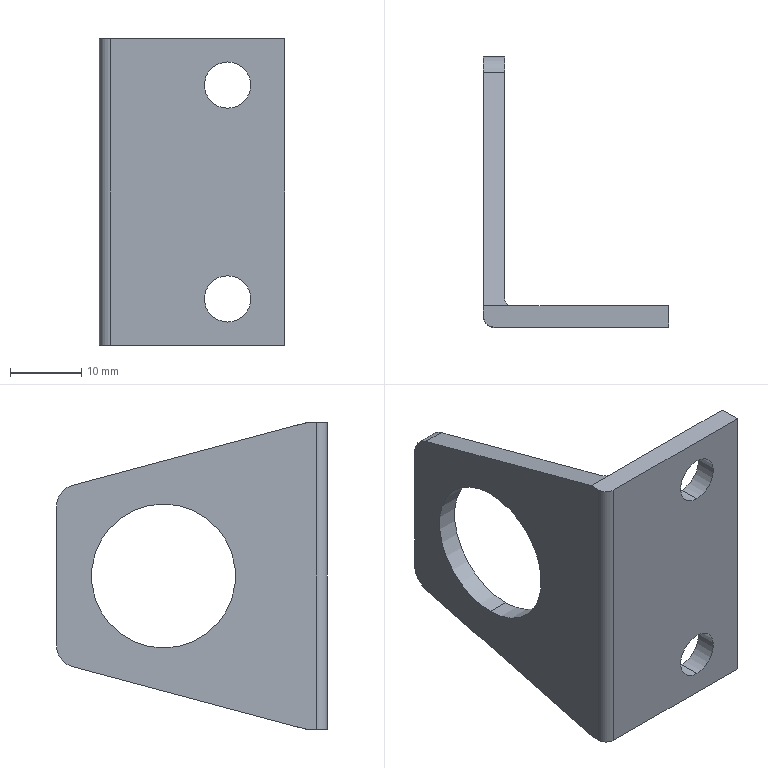Part | SolidWorks | features BaseBody 1 | 1 solid | 20 faces | box 26 x 38 x 43 mm | volume 5706 mm3 | cylinder 10 | plane 10 | commonest cylinder face diameters 6.5 x4 6 x2 20.2 x2 2 x1 3 x1
STEP:
#1=CARTESIAN_POINT('',(18.,0.,-11.75));
#2=VERTEX_POINT('',#1);
#3=CARTESIAN_POINT('',(18.,0.,-18.25));
#4=VERTEX_POINT('',#3);
#5=CARTESIAN_POINT('',(18.,0.,-15.));
#6=DIRECTION('',(0.,-1.,0.));
#7=DIRECTION('',(0.,0.,1.));
#8=AXIS2_PLACEMENT_3D('',#5,#6,#7);
#9=CIRCLE('',#8,3.25);
#10=EDGE_CURVE('',#2,#4,#9,.T.);
#11=ORIENTED_EDGE('',*,*,#10,.T.);
#12=CARTESIAN_POINT('',(18.,3.,-18.25));
#13=VERTEX_POINT('',#12);
#14=CARTESIAN_POINT('',(18.,3.,-18.25));
#15=DIRECTION('',(0.,1.,0.));
#16=VECTOR('',#15,1000.);
#17=LINE('',#14,#16);
#18=EDGE_CURVE('',#4,#13,#17,.T.);
#19=ORIENTED_EDGE('',*,*,#18,.T.);
#20=CARTESIAN_POINT('',(18.,3.,-11.75));
#21=VERTEX_POINT('',#20);
#22=CARTESIAN_POINT('',(18.,3.,-15.));
#23=DIRECTION('',(0.,-1.,0.));
#24=DIRECTION('',(0.,0.,1.));
#25=AXIS2_PLACEMENT_3D('',#22,#23,#24);
#26=CIRCLE('',#25,3.25);
#27=EDGE_CURVE('',#21,#13,#26,.T.);
#28=ORIENTED_EDGE('',*,*,#27,.F.);
#29=CARTESIAN_POINT('',(18.,3.,-11.75));
#30=DIRECTION('',(0.,1.,0.));
#31=VECTOR('',#30,1000.);
#32=LINE('',#29,#31);
#33=EDGE_CURVE('',#2,#21,#32,.T.);
#34=ORIENTED_EDGE('',*,*,#33,.F.);
#35=EDGE_LOOP('',(#11,#19,#28,#34));
#36=FACE_OUTER_BOUND('',#35,.T.);
#37=CARTESIAN_POINT('',(18.,3.,-15.));
#38=DIRECTION('',(0.,1.,0.));
#39=DIRECTION('',(0.,0.,1.));
#40=AXIS2_PLACEMENT_3D('',#37,#38,#39);
#41=CYLINDRICAL_SURFACE('',#40,3.25);
#42=ADVANCED_FACE('',(#36),#41,.F.);
#43=CARTESIAN_POINT('',(18.,0.,18.25));
#44=VERTEX_POINT('',#43);
#45=CARTESIAN_POINT('',(18.,0.,11.75));
#46=VERTEX_POINT('',#45);
#47=CARTESIAN_POINT('',(18.,0.,15.));
#48=DIRECTION('',(0.,-1.,0.));
#49=DIRECTION('',(0.,0.,1.));
#50=AXIS2_PLACEMENT_3D('',#47,#48,#49);
#51=CIRCLE('',#50,3.25);
#52=EDGE_CURVE('',#44,#46,#51,.T.);
#53=ORIENTED_EDGE('',*,*,#52,.T.);
#54=CARTESIAN_POINT('',(18.,3.,11.75));
#55=VERTEX_POINT('',#54);
#56=CARTESIAN_POINT('',(18.,3.,11.75));
#57=DIRECTION('',(0.,1.,0.));
#58=VECTOR('',#57,1000.);
#59=LINE('',#56,#58);
#60=EDGE_CURVE('',#46,#55,#59,.T.);
#61=ORIENTED_EDGE('',*,*,#60,.T.);
#62=CARTESIAN_POINT('',(18.,3.,18.25));
#63=VERTEX_POINT('',#62);
#64=CARTESIAN_POINT('',(18.,3.,15.));
#65=DIRECTION('',(0.,-1.,0.));
#66=DIRECTION('',(0.,0.,1.));
#67=AXIS2_PLACEMENT_3D('',#64,#65,#66);
#68=CIRCLE('',#67,3.25);
#69=EDGE_CURVE('',#63,#55,#68,.T.);
#70=ORIENTED_EDGE('',*,*,#69,.F.);
#71=CARTESIAN_POINT('',(18.,3.,18.25));
#72=DIRECTION('',(0.,1.,0.));
#73=VECTOR('',#72,1000.);
#74=LINE('',#71,#73);
#75=EDGE_CURVE('',#44,#63,#74,.T.);
#76=ORIENTED_EDGE('',*,*,#75,.F.);
#77=EDGE_LOOP('',(#53,#61,#70,#76));
#78=FACE_OUTER_BOUND('',#77,.T.);
#79=CARTESIAN_POINT('',(18.,3.,15.));
#80=DIRECTION('',(0.,1.,0.));
#81=DIRECTION('',(0.,0.,1.));
#82=AXIS2_PLACEMENT_3D('',#79,#80,#81);
#83=CYLINDRICAL_SURFACE('',#82,3.25);
#84=ADVANCED_FACE('',(#78),#83,.F.);
#85=CARTESIAN_POINT('',(0.,23.,-10.1));
#86=VERTEX_POINT('',#85);
#87=CARTESIAN_POINT('',(0.,23.,10.1));
#88=VERTEX_POINT('',#87);
#89=CARTESIAN_POINT('',(0.,23.,0.));
#90=DIRECTION('',(-1.,0.,0.));
#91=DIRECTION('',(0.,0.,-1.));
#92=AXIS2_PLACEMENT_3D('',#89,#90,#91);
#93=CIRCLE('',#92,10.1);
#94=EDGE_CURVE('',#86,#88,#93,.T.);
#95=ORIENTED_EDGE('',*,*,#94,.T.);
#96=CARTESIAN_POINT('',(3.,23.,10.1));
#97=VERTEX_POINT('',#96);
#98=CARTESIAN_POINT('',(26.,23.,10.1));
#99=DIRECTION('',(1.,0.,0.));
#100=VECTOR('',#99,1000.);
#101=LINE('',#98,#100);
#102=EDGE_CURVE('',#88,#97,#101,.T.);
#103=ORIENTED_EDGE('',*,*,#102,.T.);
#104=CARTESIAN_POINT('',(3.,23.,-10.1));
#105=VERTEX_POINT('',#104);
#106=CARTESIAN_POINT('',(3.,23.,0.));
#107=DIRECTION('',(-1.,0.,0.));
#108=DIRECTION('',(0.,0.,-1.));
#109=AXIS2_PLACEMENT_3D('',#106,#107,#108);
#110=CIRCLE('',#109,10.1);
#111=EDGE_CURVE('',#105,#97,#110,.T.);
#112=ORIENTED_EDGE('',*,*,#111,.F.);
#113=CARTESIAN_POINT('',(26.,23.,-10.1));
#114=DIRECTION('',(1.,0.,0.));
#115=VECTOR('',#114,1000.);
#116=LINE('',#113,#115);
#117=EDGE_CURVE('',#86,#105,#116,.T.);
#118=ORIENTED_EDGE('',*,*,#117,.F.);
#119=EDGE_LOOP('',(#95,#103,#112,#118));
#120=FACE_OUTER_BOUND('',#119,.T.);
#121=CARTESIAN_POINT('',(26.,23.,0.));
#122=DIRECTION('',(1.,0.,0.));
#123=DIRECTION('',(0.,0.,-1.));
#124=AXIS2_PLACEMENT_3D('',#121,#122,#123);
#125=CYLINDRICAL_SURFACE('',#124,10.1);
#126=ADVANCED_FACE('',(#120),#125,.F.);
#127=CARTESIAN_POINT('',(26.,0.,-21.5));
#128=VERTEX_POINT('',#127);
#129=CARTESIAN_POINT('',(1.5,0.,-21.5));
#130=VERTEX_POINT('',#129);
#131=CARTESIAN_POINT('',(26.,0.,-21.5));
#132=DIRECTION('',(-1.,0.,0.));
#133=VECTOR('',#132,1000.);
#134=LINE('',#131,#133);
#135=EDGE_CURVE('',#128,#130,#134,.T.);
#136=ORIENTED_EDGE('',*,*,#135,.F.);
#137=CARTESIAN_POINT('',(26.,0.,21.5));
#138=VERTEX_POINT('',#137);
#139=CARTESIAN_POINT('',(26.,0.,21.5));
#140=DIRECTION('',(0.,0.,-1.));
#141=VECTOR('',#140,1000.);
#142=LINE('',#139,#141);
#143=EDGE_CURVE('',#138,#128,#142,.T.);
#144=ORIENTED_EDGE('',*,*,#143,.F.);
#145=CARTESIAN_POINT('',(1.5,0.,21.5));
#146=VERTEX_POINT('',#145);
#147=CARTESIAN_POINT('',(26.,0.,21.5));
#148=DIRECTION('',(1.,0.,0.));
#149=VECTOR('',#148,1000.);
#150=LINE('',#147,#149);
#151=EDGE_CURVE('',#146,#138,#150,.T.);
#152=ORIENTED_EDGE('',*,*,#151,.F.);
#153=CARTESIAN_POINT('',(1.5,0.,21.5));
#154=DIRECTION('',(0.,0.,1.));
#155=VECTOR('',#154,1000.);
#156=LINE('',#153,#155);
#157=EDGE_CURVE('',#130,#146,#156,.T.);
#158=ORIENTED_EDGE('',*,*,#157,.F.);
#159=EDGE_LOOP('',(#136,#144,#152,#158));
#160=FACE_OUTER_BOUND('',#159,.T.);
#161=ORIENTED_EDGE('',*,*,#10,.F.);
#162=CARTESIAN_POINT('',(18.,0.,-15.));
#163=DIRECTION('',(0.,-1.,0.));
#164=DIRECTION('',(0.,0.,1.));
#165=AXIS2_PLACEMENT_3D('',#162,#163,#164);
#166=CIRCLE('',#165,3.25);
#167=EDGE_CURVE('',#4,#2,#166,.T.);
#168=ORIENTED_EDGE('',*,*,#167,.F.);
#169=EDGE_LOOP('',(#161,#168));
#170=FACE_BOUND('',#169,.T.);
#171=ORIENTED_EDGE('',*,*,#52,.F.);
#172=CARTESIAN_POINT('',(18.,0.,15.));
#173=DIRECTION('',(0.,-1.,0.));
#174=DIRECTION('',(0.,0.,1.));
#175=AXIS2_PLACEMENT_3D('',#172,#173,#174);
#176=CIRCLE('',#175,3.25);
#177=EDGE_CURVE('',#46,#44,#176,.T.);
#178=ORIENTED_EDGE('',*,*,#177,.F.);
#179=EDGE_LOOP('',(#171,#178));
#180=FACE_BOUND('',#179,.T.);
#181=CARTESIAN_POINT('',(26.,0.,21.5));
#182=DIRECTION('',(0.,1.,0.));
#183=DIRECTION('',(0.,0.,1.));
#184=AXIS2_PLACEMENT_3D('',#181,#182,#183);
#185=PLANE('',#184);
#186=ADVANCED_FACE('',(#160,#170,#180),#185,.F.);
#187=CARTESIAN_POINT('',(0.,1.5,21.5));
#188=VERTEX_POINT('',#187);
#189=CARTESIAN_POINT('',(1.5,1.5,21.5));
#190=DIRECTION('',(0.,0.,-1.));
#191=DIRECTION('',(1.,0.,0.));
#192=AXIS2_PLACEMENT_3D('',#189,#190,#191);
#193=CIRCLE('',#192,1.5);
#194=EDGE_CURVE('',#146,#188,#193,.T.);
#195=ORIENTED_EDGE('',*,*,#194,.T.);
#196=CARTESIAN_POINT('',(0.,1.5,-21.5));
#197=VERTEX_POINT('',#196);
#198=CARTESIAN_POINT('',(0.,1.5,21.5));
#199=DIRECTION('',(0.,0.,-1.));
#200=VECTOR('',#199,1000.);
#201=LINE('',#198,#200);
#202=EDGE_CURVE('',#188,#197,#201,.T.);
#203=ORIENTED_EDGE('',*,*,#202,.T.);
#204=CARTESIAN_POINT('',(1.5,1.5,-21.5));
#205=DIRECTION('',(0.,0.,1.));
#206=DIRECTION('',(1.,0.,0.));
#207=AXIS2_PLACEMENT_3D('',#204,#205,#206);
#208=CIRCLE('',#207,1.5);
#209=EDGE_CURVE('',#197,#130,#208,.T.);
#210=ORIENTED_EDGE('',*,*,#209,.T.);
#211=ORIENTED_EDGE('',*,*,#157,.T.);
#212=EDGE_LOOP('',(#195,#203,#210,#211));
#213=FACE_OUTER_BOUND('',#212,.T.);
#214=CARTESIAN_POINT('',(1.5,1.5,21.5));
#215=DIRECTION('',(0.,0.,1.));
#216=DIRECTION('',(1.,0.,0.));
#217=AXIS2_PLACEMENT_3D('',#214,#215,#216);
#218=CYLINDRICAL_SURFACE('',#217,1.5);
#219=ADVANCED_FACE('',(#213),#218,.T.);
#220=ORIENTED_EDGE('',*,*,#209,.F.);
#221=CARTESIAN_POINT('',(0.,3.,-21.5));
#222=VERTEX_POINT('',#221);
#223=CARTESIAN_POINT('',(0.,0.,-21.5));
#224=DIRECTION('',(0.,-1.,0.));
#225=VECTOR('',#224,1000.);
#226=LINE('',#223,#225);
#227=EDGE_CURVE('',#222,#197,#226,.T.);
#228=ORIENTED_EDGE('',*,*,#227,.F.);
#229=CARTESIAN_POINT('',(4.,3.,-21.5));
#230=VERTEX_POINT('',#229);
#231=CARTESIAN_POINT('',(26.,3.,-21.5));
#232=DIRECTION('',(-1.,0.,0.));
#233=VECTOR('',#232,1000.);
#234=LINE('',#231,#233);
#235=EDGE_CURVE('',#230,#222,#234,.T.);
#236=ORIENTED_EDGE('',*,*,#235,.F.);
#237=CARTESIAN_POINT('',(26.,3.,-21.5));
#238=VERTEX_POINT('',#237);
#239=CARTESIAN_POINT('',(26.,3.,-21.5));
#240=DIRECTION('',(-1.,0.,0.));
#241=VECTOR('',#240,1000.);
#242=LINE('',#239,#241);
#243=EDGE_CURVE('',#238,#230,#242,.T.);
#244=ORIENTED_EDGE('',*,*,#243,.F.);
#245=CARTESIAN_POINT('',(26.,0.,-21.5));
#246=DIRECTION('',(0.,1.,0.));
#247=VECTOR('',#246,1000.);
#248=LINE('',#245,#247);
#249=EDGE_CURVE('',#128,#238,#248,.T.);
#250=ORIENTED_EDGE('',*,*,#249,.F.);
#251=ORIENTED_EDGE('',*,*,#135,.T.);
#252=EDGE_LOOP('',(#220,#228,#236,#244,#250,#251));
#253=FACE_OUTER_BOUND('',#252,.T.);
#254=CARTESIAN_POINT('',(26.,0.,-21.5));
#255=DIRECTION('',(0.,0.,1.));
#256=DIRECTION('',(0.,-1.,0.));
#257=AXIS2_PLACEMENT_3D('',#254,#255,#256);
#258=PLANE('',#257);
#259=ADVANCED_FACE('',(#253),#258,.F.);
#260=CARTESIAN_POINT('',(26.,3.,21.5));
#261=VERTEX_POINT('',#260);
#262=CARTESIAN_POINT('',(26.,35.,21.5));
#263=DIRECTION('',(0.,-1.,0.));
#264=VECTOR('',#263,1000.);
#265=LINE('',#262,#264);
#266=EDGE_CURVE('',#261,#138,#265,.T.);
#267=ORIENTED_EDGE('',*,*,#266,.T.);
#268=ORIENTED_EDGE('',*,*,#143,.T.);
#269=ORIENTED_EDGE('',*,*,#249,.T.);
#270=CARTESIAN_POINT('',(26.,3.,-9.82));
#271=DIRECTION('',(0.,0.,1.));
#272=VECTOR('',#271,1000.);
#273=LINE('',#270,#272);
#274=EDGE_CURVE('',#238,#261,#273,.T.);
#275=ORIENTED_EDGE('',*,*,#274,.T.);
#276=EDGE_LOOP('',(#267,#268,#269,#275));
#277=FACE_OUTER_BOUND('',#276,.T.);
#278=CARTESIAN_POINT('',(26.,35.,-9.82));
#279=DIRECTION('',(1.,0.,0.));
#280=DIRECTION('',(0.,0.,-1.));
#281=AXIS2_PLACEMENT_3D('',#278,#279,#280);
#282=PLANE('',#281);
#283=ADVANCED_FACE('',(#277),#282,.T.);
#284=ORIENTED_EDGE('',*,*,#194,.F.);
#285=ORIENTED_EDGE('',*,*,#151,.T.);
#286=ORIENTED_EDGE('',*,*,#266,.F.);
#287=CARTESIAN_POINT('',(4.,3.,21.5));
#288=VERTEX_POINT('',#287);
#289=CARTESIAN_POINT('',(26.,3.,21.5));
#290=DIRECTION('',(1.,0.,0.));
#291=VECTOR('',#290,1000.);
#292=LINE('',#289,#291);
#293=EDGE_CURVE('',#288,#261,#292,.T.);
#294=ORIENTED_EDGE('',*,*,#293,.F.);
#295=CARTESIAN_POINT('',(0.,3.,21.5));
#296=VERTEX_POINT('',#295);
#297=CARTESIAN_POINT('',(26.,3.,21.5));
#298=DIRECTION('',(1.,0.,0.));
#299=VECTOR('',#298,1000.);
#300=LINE('',#297,#299);
#301=EDGE_CURVE('',#296,#288,#300,.T.);
#302=ORIENTED_EDGE('',*,*,#301,.F.);
#303=CARTESIAN_POINT('',(0.,3.,21.5));
#304=DIRECTION('',(0.,1.,0.));
#305=VECTOR('',#304,1000.);
#306=LINE('',#303,#305);
#307=EDGE_CURVE('',#188,#296,#306,.T.);
#308=ORIENTED_EDGE('',*,*,#307,.F.);
#309=EDGE_LOOP('',(#284,#285,#286,#294,#302,#308));
#310=FACE_OUTER_BOUND('',#309,.T.);
#311=CARTESIAN_POINT('',(26.,3.,21.5));
#312=DIRECTION('',(0.,0.,-1.));
#313=DIRECTION('',(-1.,0.,0.));
#314=AXIS2_PLACEMENT_3D('',#311,#312,#313);
#315=PLANE('',#314);
#316=ADVANCED_FACE('',(#310),#315,.F.);
#317=ORIENTED_EDGE('',*,*,#18,.F.);
#318=ORIENTED_EDGE('',*,*,#167,.T.);
#319=ORIENTED_EDGE('',*,*,#33,.T.);
#320=CARTESIAN_POINT('',(18.,3.,-15.));
#321=DIRECTION('',(0.,-1.,0.));
#322=DIRECTION('',(0.,0.,1.));
#323=AXIS2_PLACEMENT_3D('',#320,#321,#322);
#324=CIRCLE('',#323,3.25);
#325=EDGE_CURVE('',#13,#21,#324,.T.);
#326=ORIENTED_EDGE('',*,*,#325,.F.);
#327=EDGE_LOOP('',(#317,#318,#319,#326));
#328=FACE_OUTER_BOUND('',#327,.T.);
#329=CARTESIAN_POINT('',(18.,3.,-15.));
#330=DIRECTION('',(0.,1.,0.));
#331=DIRECTION('',(0.,0.,1.));
#332=AXIS2_PLACEMENT_3D('',#329,#330,#331);
#333=CYLINDRICAL_SURFACE('',#332,3.25);
#334=ADVANCED_FACE('',(#328),#333,.F.);
#335=ORIENTED_EDGE('',*,*,#60,.F.);
#336=ORIENTED_EDGE('',*,*,#177,.T.);
#337=ORIENTED_EDGE('',*,*,#75,.T.);
#338=CARTESIAN_POINT('',(18.,3.,15.));
#339=DIRECTION('',(0.,-1.,0.));
#340=DIRECTION('',(0.,0.,1.));
#341=AXIS2_PLACEMENT_3D('',#338,#339,#340);
#342=CIRCLE('',#341,3.25);
#343=EDGE_CURVE('',#55,#63,#342,.T.);
#344=ORIENTED_EDGE('',*,*,#343,.F.);
#345=EDGE_LOOP('',(#335,#336,#337,#344));
#346=FACE_OUTER_BOUND('',#345,.T.);
#347=CARTESIAN_POINT('',(18.,3.,15.));
#348=DIRECTION('',(0.,1.,0.));
#349=DIRECTION('',(0.,0.,1.));
#350=AXIS2_PLACEMENT_3D('',#347,#348,#349);
#351=CYLINDRICAL_SURFACE('',#350,3.25);
#352=ADVANCED_FACE('',(#346),#351,.F.);
#353=ORIENTED_EDGE('',*,*,#202,.F.);
#354=ORIENTED_EDGE('',*,*,#307,.T.);
#355=CARTESIAN_POINT('',(0.,35.776,12.718));
#356=VERTEX_POINT('',#355);
#357=CARTESIAN_POINT('',(0.,35.776,12.718));
#358=DIRECTION('',(0.,-0.9659,0.2588));
#359=VECTOR('',#358,1000.);
#360=LINE('',#357,#359);
#361=EDGE_CURVE('',#356,#296,#360,.T.);
#362=ORIENTED_EDGE('',*,*,#361,.F.);
#363=CARTESIAN_POINT('',(0.,38.,9.82));
#364=VERTEX_POINT('',#363);
#365=CARTESIAN_POINT('',(0.,35.,9.82));
#366=DIRECTION('',(1.,0.,0.));
#367=DIRECTION('',(0.,0.,-1.));
#368=AXIS2_PLACEMENT_3D('',#365,#366,#367);
#369=CIRCLE('',#368,3.);
#370=EDGE_CURVE('',#364,#356,#369,.T.);
#371=ORIENTED_EDGE('',*,*,#370,.F.);
#372=CARTESIAN_POINT('',(0.,38.,-9.82));
#373=VERTEX_POINT('',#372);
#374=CARTESIAN_POINT('',(0.,38.,-9.82));
#375=DIRECTION('',(0.,0.,1.));
#376=VECTOR('',#375,1000.);
#377=LINE('',#374,#376);
#378=EDGE_CURVE('',#373,#364,#377,.T.);
#379=ORIENTED_EDGE('',*,*,#378,.F.);
#380=CARTESIAN_POINT('',(0.,35.776,-12.718));
#381=VERTEX_POINT('',#380);
#382=CARTESIAN_POINT('',(0.,35.,-9.82));
#383=DIRECTION('',(1.,0.,0.));
#384=DIRECTION('',(0.,0.,-1.));
#385=AXIS2_PLACEMENT_3D('',#382,#383,#384);
#386=CIRCLE('',#385,3.);
#387=EDGE_CURVE('',#381,#373,#386,.T.);
#388=ORIENTED_EDGE('',*,*,#387,.F.);
#389=CARTESIAN_POINT('',(0.,3.,-21.5));
#390=DIRECTION('',(0.,0.9659,0.2588));
#391=VECTOR('',#390,1000.);
#392=LINE('',#389,#391);
#393=EDGE_CURVE('',#222,#381,#392,.T.);
#394=ORIENTED_EDGE('',*,*,#393,.F.);
#395=ORIENTED_EDGE('',*,*,#227,.T.);
#396=EDGE_LOOP('',(#353,#354,#362,#371,#379,#388,#394,#395));
#397=FACE_OUTER_BOUND('',#396,.T.);
#398=ORIENTED_EDGE('',*,*,#94,.F.);
#399=CARTESIAN_POINT('',(0.,23.,0.));
#400=DIRECTION('',(-1.,0.,0.));
#401=DIRECTION('',(0.,0.,-1.));
#402=AXIS2_PLACEMENT_3D('',#399,#400,#401);
#403=CIRCLE('',#402,10.1);
#404=EDGE_CURVE('',#88,#86,#403,.T.);
#405=ORIENTED_EDGE('',*,*,#404,.F.);
#406=EDGE_LOOP('',(#398,#405));
#407=FACE_BOUND('',#406,.T.);
#408=CARTESIAN_POINT('',(0.,35.,-9.82));
#409=DIRECTION('',(1.,0.,0.));
#410=DIRECTION('',(0.,0.,-1.));
#411=AXIS2_PLACEMENT_3D('',#408,#409,#410);
#412=PLANE('',#411);
#413=ADVANCED_FACE('',(#397,#407),#412,.F.);
#414=CARTESIAN_POINT('',(3.,4.,-21.232));
#415=VERTEX_POINT('',#414);
#416=CARTESIAN_POINT('',(3.,4.,-21.232));
#417=CARTESIAN_POINT('',(3.,3.414,-21.389));
#418=CARTESIAN_POINT('',(3.414,3.,-21.5));
#419=CARTESIAN_POINT('',(4.,3.,-21.5));
#420=(BOUNDED_CURVE()B_SPLINE_CURVE(3,(#416,#417,#418,#419),.UNSPECIFIED.,.F.,.F.)B_SPLINE_CURVE_WITH_KNOTS((4,4),(1.571,3.142),.UNSPECIFIED.)CURVE()GEOMETRIC_REPRESENTATION_ITEM()RATIONAL_B_SPLINE_CURVE((1.,0.8047,0.8047,1.))REPRESENTATION_ITEM(''));
#421=EDGE_CURVE('',#415,#230,#420,.T.);
#422=ORIENTED_EDGE('',*,*,#421,.T.);
#423=ORIENTED_EDGE('',*,*,#235,.T.);
#424=ORIENTED_EDGE('',*,*,#393,.T.);
#425=CARTESIAN_POINT('',(3.,35.776,-12.718));
#426=VERTEX_POINT('',#425);
#427=CARTESIAN_POINT('',(26.,35.776,-12.718));
#428=DIRECTION('',(-1.,0.,0.));
#429=VECTOR('',#428,1000.);
#430=LINE('',#427,#429);
#431=EDGE_CURVE('',#426,#381,#430,.T.);
#432=ORIENTED_EDGE('',*,*,#431,.F.);
#433=CARTESIAN_POINT('',(3.,3.,-21.5));
#434=DIRECTION('',(0.,0.9659,0.2588));
#435=VECTOR('',#434,1000.);
#436=LINE('',#433,#435);
#437=EDGE_CURVE('',#415,#426,#436,.T.);
#438=ORIENTED_EDGE('',*,*,#437,.F.);
#439=EDGE_LOOP('',(#422,#423,#424,#432,#438));
#440=FACE_OUTER_BOUND('',#439,.T.);
#441=CARTESIAN_POINT('',(26.,3.,-21.5));
#442=DIRECTION('',(0.,-0.2588,0.9659));
#443=DIRECTION('',(0.,-0.9659,-0.2588));
#444=AXIS2_PLACEMENT_3D('',#441,#442,#443);
#445=PLANE('',#444);
#446=ADVANCED_FACE('',(#440),#445,.F.);
#447=ORIENTED_EDGE('',*,*,#293,.T.);
#448=ORIENTED_EDGE('',*,*,#274,.F.);
#449=ORIENTED_EDGE('',*,*,#243,.T.);
#450=CARTESIAN_POINT('',(4.,3.,21.5));
#451=DIRECTION('',(0.,0.,1.));
#452=VECTOR('',#451,1000.);
#453=LINE('',#450,#452);
#454=EDGE_CURVE('',#230,#288,#453,.T.);
#455=ORIENTED_EDGE('',*,*,#454,.T.);
#456=EDGE_LOOP('',(#447,#448,#449,#455));
#457=FACE_OUTER_BOUND('',#456,.T.);
#458=ORIENTED_EDGE('',*,*,#27,.T.);
#459=ORIENTED_EDGE('',*,*,#325,.T.);
#460=EDGE_LOOP('',(#458,#459));
#461=FACE_BOUND('',#460,.T.);
#462=ORIENTED_EDGE('',*,*,#69,.T.);
#463=ORIENTED_EDGE('',*,*,#343,.T.);
#464=EDGE_LOOP('',(#462,#463));
#465=FACE_BOUND('',#464,.T.);
#466=CARTESIAN_POINT('',(4.,3.,21.5));
#467=DIRECTION('',(0.,1.,0.));
#468=DIRECTION('',(0.,0.,1.));
#469=AXIS2_PLACEMENT_3D('',#466,#467,#468);
#470=PLANE('',#469);
#471=ADVANCED_FACE('',(#457,#461,#465),#470,.T.);
#472=CARTESIAN_POINT('',(3.,35.776,12.718));
#473=VERTEX_POINT('',#472);
#474=CARTESIAN_POINT('',(26.,35.776,12.718));
#475=DIRECTION('',(1.,0.,0.));
#476=VECTOR('',#475,1000.);
#477=LINE('',#474,#476);
#478=EDGE_CURVE('',#356,#473,#477,.T.);
#479=ORIENTED_EDGE('',*,*,#478,.F.);
#480=ORIENTED_EDGE('',*,*,#361,.T.);
#481=ORIENTED_EDGE('',*,*,#301,.T.);
#482=CARTESIAN_POINT('',(3.,4.,21.232));
#483=VERTEX_POINT('',#482);
#484=CARTESIAN_POINT('',(3.,4.,21.232));
#485=CARTESIAN_POINT('',(3.,3.414,21.389));
#486=CARTESIAN_POINT('',(3.414,3.,21.5));
#487=CARTESIAN_POINT('',(4.,3.,21.5));
#488=(BOUNDED_CURVE()B_SPLINE_CURVE(3,(#484,#485,#486,#487),.UNSPECIFIED.,.F.,.F.)B_SPLINE_CURVE_WITH_KNOTS((4,4),(4.712,6.283),.UNSPECIFIED.)CURVE()GEOMETRIC_REPRESENTATION_ITEM()RATIONAL_B_SPLINE_CURVE((1.,0.8047,0.8047,1.))REPRESENTATION_ITEM(''));
#489=EDGE_CURVE('',#483,#288,#488,.T.);
#490=ORIENTED_EDGE('',*,*,#489,.F.);
#491=CARTESIAN_POINT('',(3.,35.776,12.718));
#492=DIRECTION('',(0.,-0.9659,0.2588));
#493=VECTOR('',#492,1000.);
#494=LINE('',#491,#493);
#495=EDGE_CURVE('',#473,#483,#494,.T.);
#496=ORIENTED_EDGE('',*,*,#495,.F.);
#497=EDGE_LOOP('',(#479,#480,#481,#490,#496));
#498=FACE_OUTER_BOUND('',#497,.T.);
#499=CARTESIAN_POINT('',(26.,35.776,12.718));
#500=DIRECTION('',(0.,-0.2588,-0.9659));
#501=DIRECTION('',(0.,0.9659,-0.2588));
#502=AXIS2_PLACEMENT_3D('',#499,#500,#501);
#503=PLANE('',#502);
#504=ADVANCED_FACE('',(#498),#503,.F.);
#505=ORIENTED_EDGE('',*,*,#370,.T.);
#506=ORIENTED_EDGE('',*,*,#478,.T.);
#507=CARTESIAN_POINT('',(3.,38.,9.82));
#508=VERTEX_POINT('',#507);
#509=CARTESIAN_POINT('',(3.,35.,9.82));
#510=DIRECTION('',(-1.,0.,0.));
#511=DIRECTION('',(0.,0.,-1.));
#512=AXIS2_PLACEMENT_3D('',#509,#510,#511);
#513=CIRCLE('',#512,3.);
#514=EDGE_CURVE('',#473,#508,#513,.T.);
#515=ORIENTED_EDGE('',*,*,#514,.T.);
#516=CARTESIAN_POINT('',(26.,38.,9.82));
#517=DIRECTION('',(-1.,0.,0.));
#518=VECTOR('',#517,1000.);
#519=LINE('',#516,#518);
#520=EDGE_CURVE('',#508,#364,#519,.T.);
#521=ORIENTED_EDGE('',*,*,#520,.T.);
#522=EDGE_LOOP('',(#505,#506,#515,#521));
#523=FACE_OUTER_BOUND('',#522,.T.);
#524=CARTESIAN_POINT('',(26.,35.,9.82));
#525=DIRECTION('',(1.,0.,0.));
#526=DIRECTION('',(0.,0.,-1.));
#527=AXIS2_PLACEMENT_3D('',#524,#525,#526);
#528=CYLINDRICAL_SURFACE('',#527,3.);
#529=ADVANCED_FACE('',(#523),#528,.T.);
#530=CARTESIAN_POINT('',(3.,38.,-9.82));
#531=VERTEX_POINT('',#530);
#532=CARTESIAN_POINT('',(26.,38.,-9.82));
#533=DIRECTION('',(1.,0.,0.));
#534=VECTOR('',#533,1000.);
#535=LINE('',#532,#534);
#536=EDGE_CURVE('',#373,#531,#535,.T.);
#537=ORIENTED_EDGE('',*,*,#536,.F.);
#538=ORIENTED_EDGE('',*,*,#378,.T.);
#539=ORIENTED_EDGE('',*,*,#520,.F.);
#540=CARTESIAN_POINT('',(3.,38.,-9.82));
#541=DIRECTION('',(0.,0.,1.));
#542=VECTOR('',#541,1000.);
#543=LINE('',#540,#542);
#544=EDGE_CURVE('',#531,#508,#543,.T.);
#545=ORIENTED_EDGE('',*,*,#544,.F.);
#546=EDGE_LOOP('',(#537,#538,#539,#545));
#547=FACE_OUTER_BOUND('',#546,.T.);
#548=CARTESIAN_POINT('',(26.,38.,-9.82));
#549=DIRECTION('',(0.,-1.,0.));
#550=DIRECTION('',(0.,0.,-1.));
#551=AXIS2_PLACEMENT_3D('',#548,#549,#550);
#552=PLANE('',#551);
#553=ADVANCED_FACE('',(#547),#552,.F.);
#554=ORIENTED_EDGE('',*,*,#387,.T.);
#555=ORIENTED_EDGE('',*,*,#536,.T.);
#556=CARTESIAN_POINT('',(3.,35.,-9.82));
#557=DIRECTION('',(-1.,0.,0.));
#558=DIRECTION('',(0.,0.,-1.));
#559=AXIS2_PLACEMENT_3D('',#556,#557,#558);
#560=CIRCLE('',#559,3.);
#561=EDGE_CURVE('',#531,#426,#560,.T.);
#562=ORIENTED_EDGE('',*,*,#561,.T.);
#563=ORIENTED_EDGE('',*,*,#431,.T.);
#564=EDGE_LOOP('',(#554,#555,#562,#563));
#565=FACE_OUTER_BOUND('',#564,.T.);
#566=CARTESIAN_POINT('',(26.,35.,-9.82));
#567=DIRECTION('',(1.,0.,0.));
#568=DIRECTION('',(0.,0.,-1.));
#569=AXIS2_PLACEMENT_3D('',#566,#567,#568);
#570=CYLINDRICAL_SURFACE('',#569,3.);
#571=ADVANCED_FACE('',(#565),#570,.T.);
#572=ORIENTED_EDGE('',*,*,#102,.F.);
#573=ORIENTED_EDGE('',*,*,#404,.T.);
#574=ORIENTED_EDGE('',*,*,#117,.T.);
#575=CARTESIAN_POINT('',(3.,23.,0.));
#576=DIRECTION('',(-1.,0.,0.));
#577=DIRECTION('',(0.,0.,-1.));
#578=AXIS2_PLACEMENT_3D('',#575,#576,#577);
#579=CIRCLE('',#578,10.1);
#580=EDGE_CURVE('',#97,#105,#579,.T.);
#581=ORIENTED_EDGE('',*,*,#580,.F.);
#582=EDGE_LOOP('',(#572,#573,#574,#581));
#583=FACE_OUTER_BOUND('',#582,.T.);
#584=CARTESIAN_POINT('',(26.,23.,0.));
#585=DIRECTION('',(1.,0.,0.));
#586=DIRECTION('',(0.,0.,-1.));
#587=AXIS2_PLACEMENT_3D('',#584,#585,#586);
#588=CYLINDRICAL_SURFACE('',#587,10.1);
#589=ADVANCED_FACE('',(#583),#588,.F.);
#590=ORIENTED_EDGE('',*,*,#495,.T.);
#591=CARTESIAN_POINT('',(3.,4.,21.5));
#592=DIRECTION('',(0.,0.,-1.));
#593=VECTOR('',#592,1000.);
#594=LINE('',#591,#593);
#595=EDGE_CURVE('',#483,#415,#594,.T.);
#596=ORIENTED_EDGE('',*,*,#595,.T.);
#597=ORIENTED_EDGE('',*,*,#437,.T.);
#598=ORIENTED_EDGE('',*,*,#561,.F.);
#599=ORIENTED_EDGE('',*,*,#544,.T.);
#600=ORIENTED_EDGE('',*,*,#514,.F.);
#601=EDGE_LOOP('',(#590,#596,#597,#598,#599,#600));
#602=FACE_OUTER_BOUND('',#601,.T.);
#603=ORIENTED_EDGE('',*,*,#111,.T.);
#604=ORIENTED_EDGE('',*,*,#580,.T.);
#605=EDGE_LOOP('',(#603,#604));
#606=FACE_BOUND('',#605,.T.);
#607=CARTESIAN_POINT('',(3.,38.,21.5));
#608=DIRECTION('',(1.,0.,0.));
#609=DIRECTION('',(0.,0.,-1.));
#610=AXIS2_PLACEMENT_3D('',#607,#608,#609);
#611=PLANE('',#610);
#612=ADVANCED_FACE('',(#602,#606),#611,.T.);
#613=ORIENTED_EDGE('',*,*,#454,.F.);
#614=ORIENTED_EDGE('',*,*,#421,.F.);
#615=ORIENTED_EDGE('',*,*,#595,.F.);
#616=ORIENTED_EDGE('',*,*,#489,.T.);
#617=EDGE_LOOP('',(#613,#614,#615,#616));
#618=FACE_OUTER_BOUND('',#617,.T.);
#619=CARTESIAN_POINT('',(4.,4.,21.5));
#620=DIRECTION('',(0.,0.,1.));
#621=DIRECTION('',(1.,0.,0.));
#622=AXIS2_PLACEMENT_3D('',#619,#620,#621);
#623=CYLINDRICAL_SURFACE('',#622,1.);
#624=ADVANCED_FACE('',(#618),#623,.F.);
#625=CLOSED_SHELL('',(#42,#84,#126,#186,#219,#259,#283,#316,#334,#352,#413,#446,#471,#504,#529,#553,#571,#589,#612,#624));
#626=MANIFOLD_SOLID_BREP('',#625);
#627=CARTESIAN_POINT('',(0.,0.,0.));
#628=DIRECTION('',(0.,0.,1.));
#629=DIRECTION('',(1.,0.,0.));
#630=AXIS2_PLACEMENT_3D('',#627,#628,#629);
#631=(LENGTH_UNIT()NAMED_UNIT(*)SI_UNIT(.MILLI.,.METRE.));
#632=UNCERTAINTY_MEASURE_WITH_UNIT(LENGTH_MEASURE(0.00001),#631,'','');
#633=(NAMED_UNIT(*)PLANE_ANGLE_UNIT()SI_UNIT($,.RADIAN.));
#634=(NAMED_UNIT(*)SI_UNIT($,.STERADIAN.)SOLID_ANGLE_UNIT());
#635=(GEOMETRIC_REPRESENTATION_CONTEXT(3)GLOBAL_UNCERTAINTY_ASSIGNED_CONTEXT((#632))GLOBAL_UNIT_ASSIGNED_CONTEXT((#631,#633,#634))REPRESENTATION_CONTEXT('',''));
#636=ADVANCED_BREP_SHAPE_REPRESENTATION('',(#626,#630),#635);